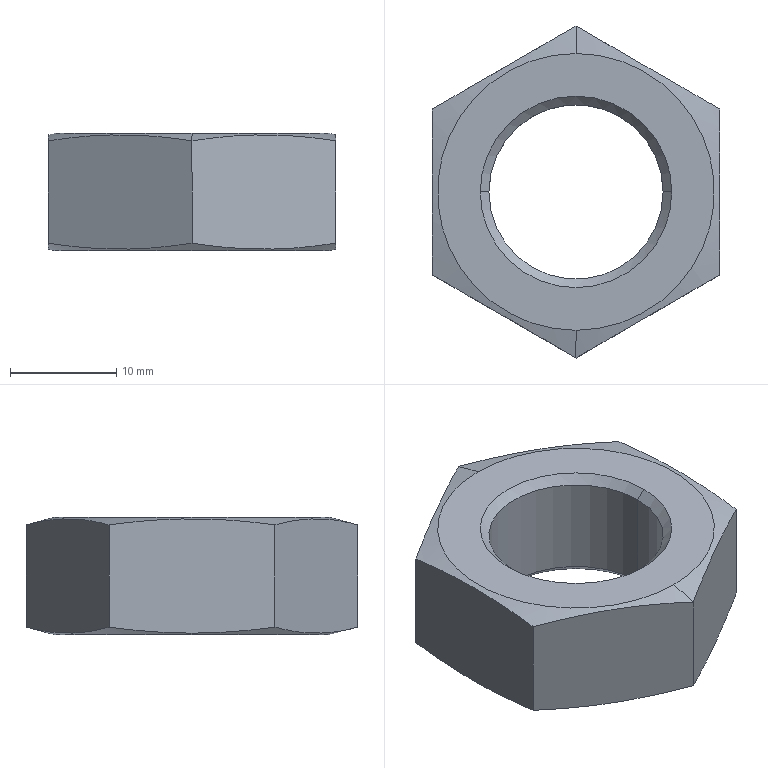Part | SolidWorks | features BaseBody 1 | 1 solid | 18 faces | box 27 x 31.177 x 11 mm | volume 4552 mm3 | cone 8 | plane 8 | cylinder 2 | commonest cylinder face diameters 16.376 x2
STEP:
#1=CARTESIAN_POINT('',(8.188,0.,4.688));
#2=VERTEX_POINT('',#1);
#3=CARTESIAN_POINT('',(-8.188,0.,4.688));
#4=VERTEX_POINT('',#3);
#5=CARTESIAN_POINT('',(0.,0.,4.688));
#6=DIRECTION('',(0.,0.,-1.));
#7=DIRECTION('',(-1.,0.,0.));
#8=AXIS2_PLACEMENT_3D('',#5,#6,#7);
#9=CIRCLE('',#8,8.188);
#10=EDGE_CURVE('',#2,#4,#9,.T.);
#11=ORIENTED_EDGE('',*,*,#10,.F.);
#12=CARTESIAN_POINT('',(8.188,0.,-4.688));
#13=VERTEX_POINT('',#12);
#14=CARTESIAN_POINT('',(8.188,0.,-5.5));
#15=DIRECTION('',(0.,0.,-1.));
#16=VECTOR('',#15,1000.);
#17=LINE('',#14,#16);
#18=EDGE_CURVE('',#2,#13,#17,.T.);
#19=ORIENTED_EDGE('',*,*,#18,.T.);
#20=CARTESIAN_POINT('',(-8.188,0.,-4.688));
#21=VERTEX_POINT('',#20);
#22=CARTESIAN_POINT('',(0.,0.,-4.688));
#23=DIRECTION('',(0.,0.,1.));
#24=DIRECTION('',(-1.,0.,0.));
#25=AXIS2_PLACEMENT_3D('',#22,#23,#24);
#26=CIRCLE('',#25,8.188);
#27=EDGE_CURVE('',#21,#13,#26,.T.);
#28=ORIENTED_EDGE('',*,*,#27,.F.);
#29=CARTESIAN_POINT('',(-8.188,0.,-5.5));
#30=DIRECTION('',(0.,0.,-1.));
#31=VECTOR('',#30,1000.);
#32=LINE('',#29,#31);
#33=EDGE_CURVE('',#4,#21,#32,.T.);
#34=ORIENTED_EDGE('',*,*,#33,.F.);
#35=EDGE_LOOP('',(#11,#19,#28,#34));
#36=FACE_OUTER_BOUND('',#35,.T.);
#37=CARTESIAN_POINT('',(0.,0.,-5.5));
#38=DIRECTION('',(0.,0.,-1.));
#39=DIRECTION('',(-1.,0.,0.));
#40=AXIS2_PLACEMENT_3D('',#37,#38,#39);
#41=CYLINDRICAL_SURFACE('',#40,8.188);
#42=ADVANCED_FACE('',(#36),#41,.F.);
#43=ORIENTED_EDGE('',*,*,#10,.T.);
#44=CARTESIAN_POINT('',(-9.,0.,5.5));
#45=VERTEX_POINT('',#44);
#46=CARTESIAN_POINT('',(-9.,0.,5.5));
#47=DIRECTION('',(-0.7071,0.,0.7071));
#48=VECTOR('',#47,1000.);
#49=LINE('',#46,#48);
#50=EDGE_CURVE('',#4,#45,#49,.T.);
#51=ORIENTED_EDGE('',*,*,#50,.T.);
#52=CARTESIAN_POINT('',(9.,0.,5.5));
#53=VERTEX_POINT('',#52);
#54=CARTESIAN_POINT('',(0.,0.,5.5));
#55=DIRECTION('',(0.,0.,-1.));
#56=DIRECTION('',(1.,0.,0.));
#57=AXIS2_PLACEMENT_3D('',#54,#55,#56);
#58=CIRCLE('',#57,9.);
#59=EDGE_CURVE('',#53,#45,#58,.T.);
#60=ORIENTED_EDGE('',*,*,#59,.F.);
#61=CARTESIAN_POINT('',(9.,0.,5.5));
#62=DIRECTION('',(0.7071,0.,0.7071));
#63=VECTOR('',#62,1000.);
#64=LINE('',#61,#63);
#65=EDGE_CURVE('',#2,#53,#64,.T.);
#66=ORIENTED_EDGE('',*,*,#65,.F.);
#67=EDGE_LOOP('',(#43,#51,#60,#66));
#68=FACE_OUTER_BOUND('',#67,.T.);
#69=CARTESIAN_POINT('',(0.,0.,5.5));
#70=DIRECTION('',(0.,0.,1.));
#71=DIRECTION('',(1.,0.,0.));
#72=AXIS2_PLACEMENT_3D('',#69,#70,#71);
#73=CONICAL_SURFACE('',#72,9.,0.7854);
#74=ADVANCED_FACE('',(#68),#73,.F.);
#75=ORIENTED_EDGE('',*,*,#27,.T.);
#76=CARTESIAN_POINT('',(9.,0.,-5.5));
#77=VERTEX_POINT('',#76);
#78=CARTESIAN_POINT('',(9.,0.,-5.5));
#79=DIRECTION('',(0.7071,0.,-0.7071));
#80=VECTOR('',#79,1000.);
#81=LINE('',#78,#80);
#82=EDGE_CURVE('',#13,#77,#81,.T.);
#83=ORIENTED_EDGE('',*,*,#82,.T.);
#84=CARTESIAN_POINT('',(-9.,0.,-5.5));
#85=VERTEX_POINT('',#84);
#86=CARTESIAN_POINT('',(0.,0.,-5.5));
#87=DIRECTION('',(0.,0.,1.));
#88=DIRECTION('',(-1.,0.,0.));
#89=AXIS2_PLACEMENT_3D('',#86,#87,#88);
#90=CIRCLE('',#89,9.);
#91=EDGE_CURVE('',#85,#77,#90,.T.);
#92=ORIENTED_EDGE('',*,*,#91,.F.);
#93=CARTESIAN_POINT('',(-9.,0.,-5.5));
#94=DIRECTION('',(-0.7071,0.,-0.7071));
#95=VECTOR('',#94,1000.);
#96=LINE('',#93,#95);
#97=EDGE_CURVE('',#21,#85,#96,.T.);
#98=ORIENTED_EDGE('',*,*,#97,.F.);
#99=EDGE_LOOP('',(#75,#83,#92,#98));
#100=FACE_OUTER_BOUND('',#99,.T.);
#101=CARTESIAN_POINT('',(0.,0.,-5.5));
#102=DIRECTION('',(0.,0.,-1.));
#103=DIRECTION('',(-1.,0.,0.));
#104=AXIS2_PLACEMENT_3D('',#101,#102,#103);
#105=CONICAL_SURFACE('',#104,9.,0.7854);
#106=ADVANCED_FACE('',(#100),#105,.F.);
#107=CARTESIAN_POINT('',(0.,-13.,5.5));
#108=VERTEX_POINT('',#107);
#109=CARTESIAN_POINT('',(0.,13.,5.5));
#110=VERTEX_POINT('',#109);
#111=CARTESIAN_POINT('',(0.,0.,5.5));
#112=DIRECTION('',(0.,0.,1.));
#113=DIRECTION('',(0.,1.,0.));
#114=AXIS2_PLACEMENT_3D('',#111,#112,#113);
#115=CIRCLE('',#114,13.);
#116=EDGE_CURVE('',#108,#110,#115,.T.);
#117=ORIENTED_EDGE('',*,*,#116,.F.);
#118=CARTESIAN_POINT('',(-0.000000051,-15.588,4.806));
#119=VERTEX_POINT('',#118);
#120=CARTESIAN_POINT('',(0.,-15.604,4.802));
#121=DIRECTION('',(0.,-0.9659,-0.2588));
#122=VECTOR('',#121,1000.);
#123=LINE('',#120,#122);
#124=EDGE_CURVE('',#108,#119,#123,.T.);
#125=ORIENTED_EDGE('',*,*,#124,.T.);
#126=CARTESIAN_POINT('',(13.5,-7.794,4.806));
#127=VERTEX_POINT('',#126);
#128=CARTESIAN_POINT('',(-0.000000051,-15.588,4.806));
#129=CARTESIAN_POINT('',(1.125,-14.939,4.98));
#130=CARTESIAN_POINT('',(2.25,-14.289,5.122));
#131=CARTESIAN_POINT('',(4.5,-12.99,5.315));
#132=CARTESIAN_POINT('',(6.75,-11.691,5.417));
#133=CARTESIAN_POINT('',(9.,-10.392,5.315));
#134=CARTESIAN_POINT('',(11.25,-9.093,5.122));
#135=CARTESIAN_POINT('',(12.375,-8.444,4.98));
#136=CARTESIAN_POINT('',(13.5,-7.794,4.806));
#137=B_SPLINE_CURVE_WITH_KNOTS('',3,(#128,#129,#130,#131,#132,#133,#134,#135,#136),.UNSPECIFIED.,.F.,.F.,(4,2,1,2,4),(0.,0.003897,0.007794,0.01169,0.01559),.UNSPECIFIED.);
#138=EDGE_CURVE('',#119,#127,#137,.T.);
#139=ORIENTED_EDGE('',*,*,#138,.T.);
#140=CARTESIAN_POINT('',(13.5,7.794,4.806));
#141=VERTEX_POINT('',#140);
#142=CARTESIAN_POINT('',(13.5,-7.794,4.806));
#143=CARTESIAN_POINT('',(13.5,-6.495,4.98));
#144=CARTESIAN_POINT('',(13.5,-5.196,5.122));
#145=CARTESIAN_POINT('',(13.5,-2.598,5.315));
#146=CARTESIAN_POINT('',(13.5,-0.000000076,5.417));
#147=CARTESIAN_POINT('',(13.5,2.598,5.315));
#148=CARTESIAN_POINT('',(13.5,5.196,5.122));
#149=CARTESIAN_POINT('',(13.5,6.495,4.98));
#150=CARTESIAN_POINT('',(13.5,7.794,4.806));
#151=B_SPLINE_CURVE_WITH_KNOTS('',3,(#142,#143,#144,#145,#146,#147,#148,#149,#150),.UNSPECIFIED.,.F.,.F.,(4,2,1,2,4),(0.,0.003897,0.007794,0.01169,0.01559),.UNSPECIFIED.);
#152=EDGE_CURVE('',#127,#141,#151,.T.);
#153=ORIENTED_EDGE('',*,*,#152,.T.);
#154=CARTESIAN_POINT('',(0.000000006,15.588,4.806));
#155=VERTEX_POINT('',#154);
#156=CARTESIAN_POINT('',(13.5,7.794,4.806));
#157=CARTESIAN_POINT('',(12.375,8.444,4.98));
#158=CARTESIAN_POINT('',(11.25,9.093,5.122));
#159=CARTESIAN_POINT('',(9.,10.392,5.315));
#160=CARTESIAN_POINT('',(6.75,11.691,5.417));
#161=CARTESIAN_POINT('',(4.5,12.99,5.315));
#162=CARTESIAN_POINT('',(2.25,14.289,5.122));
#163=CARTESIAN_POINT('',(1.125,14.939,4.98));
#164=CARTESIAN_POINT('',(0.000000006,15.588,4.806));
#165=B_SPLINE_CURVE_WITH_KNOTS('',3,(#156,#157,#158,#159,#160,#161,#162,#163,#164),.UNSPECIFIED.,.F.,.F.,(4,2,1,2,4),(0.,0.003897,0.007794,0.01169,0.01559),.UNSPECIFIED.);
#166=EDGE_CURVE('',#141,#155,#165,.T.);
#167=ORIENTED_EDGE('',*,*,#166,.T.);
#168=CARTESIAN_POINT('',(0.,15.604,4.802));
#169=DIRECTION('',(0.,0.9659,-0.2588));
#170=VECTOR('',#169,1000.);
#171=LINE('',#168,#170);
#172=EDGE_CURVE('',#110,#155,#171,.T.);
#173=ORIENTED_EDGE('',*,*,#172,.F.);
#174=EDGE_LOOP('',(#117,#125,#139,#153,#167,#173));
#175=FACE_OUTER_BOUND('',#174,.T.);
#176=CARTESIAN_POINT('',(0.,0.,4.802));
#177=DIRECTION('',(0.,0.,-1.));
#178=DIRECTION('',(0.,1.,0.));
#179=AXIS2_PLACEMENT_3D('',#176,#177,#178);
#180=CONICAL_SURFACE('',#179,15.604,1.309);
#181=ADVANCED_FACE('',(#175),#180,.T.);
#182=CARTESIAN_POINT('',(-13.,0.,-5.5));
#183=VERTEX_POINT('',#182);
#184=CARTESIAN_POINT('',(13.,0.,-5.5));
#185=VERTEX_POINT('',#184);
#186=CARTESIAN_POINT('',(0.,0.,-5.5));
#187=DIRECTION('',(0.,0.,-1.));
#188=DIRECTION('',(1.,0.,0.));
#189=AXIS2_PLACEMENT_3D('',#186,#187,#188);
#190=CIRCLE('',#189,13.);
#191=EDGE_CURVE('',#183,#185,#190,.T.);
#192=ORIENTED_EDGE('',*,*,#191,.F.);
#193=CARTESIAN_POINT('',(-13.5,0.,-5.366));
#194=VERTEX_POINT('',#193);
#195=CARTESIAN_POINT('',(-15.604,0.,-4.802));
#196=DIRECTION('',(-0.9659,0.,0.2588));
#197=VECTOR('',#196,1000.);
#198=LINE('',#195,#197);
#199=EDGE_CURVE('',#183,#194,#198,.T.);
#200=ORIENTED_EDGE('',*,*,#199,.T.);
#201=CARTESIAN_POINT('',(-13.5,7.794,-4.806));
#202=VERTEX_POINT('',#201);
#203=CARTESIAN_POINT('',(-13.5,0.,-5.366));
#204=CARTESIAN_POINT('',(-13.5,1.299,-5.366));
#205=CARTESIAN_POINT('',(-13.5,2.598,-5.315));
#206=CARTESIAN_POINT('',(-13.5,5.196,-5.122));
#207=CARTESIAN_POINT('',(-13.5,6.495,-4.98));
#208=CARTESIAN_POINT('',(-13.5,7.794,-4.806));
#209=B_SPLINE_CURVE_WITH_KNOTS('',3,(#203,#204,#205,#206,#207,#208),.UNSPECIFIED.,.F.,.F.,(4,2,4),(0.007794,0.01169,0.01559),.UNSPECIFIED.);
#210=EDGE_CURVE('',#194,#202,#209,.T.);
#211=ORIENTED_EDGE('',*,*,#210,.T.);
#212=CARTESIAN_POINT('',(-0.000000051,15.588,-4.806));
#213=VERTEX_POINT('',#212);
#214=CARTESIAN_POINT('',(-13.5,7.794,-4.806));
#215=CARTESIAN_POINT('',(-12.375,8.444,-4.98));
#216=CARTESIAN_POINT('',(-11.25,9.093,-5.122));
#217=CARTESIAN_POINT('',(-9.,10.392,-5.315));
#218=CARTESIAN_POINT('',(-6.75,11.691,-5.417));
#219=CARTESIAN_POINT('',(-4.5,12.99,-5.315));
#220=CARTESIAN_POINT('',(-2.25,14.289,-5.122));
#221=CARTESIAN_POINT('',(-1.125,14.939,-4.98));
#222=CARTESIAN_POINT('',(-0.000000051,15.588,-4.806));
#223=B_SPLINE_CURVE_WITH_KNOTS('',3,(#214,#215,#216,#217,#218,#219,#220,#221,#222),.UNSPECIFIED.,.F.,.F.,(4,2,1,2,4),(0.,0.003897,0.007794,0.01169,0.01559),.UNSPECIFIED.);
#224=EDGE_CURVE('',#202,#213,#223,.T.);
#225=ORIENTED_EDGE('',*,*,#224,.T.);
#226=CARTESIAN_POINT('',(13.5,7.794,-4.806));
#227=VERTEX_POINT('',#226);
#228=CARTESIAN_POINT('',(-0.000000051,15.588,-4.806));
#229=CARTESIAN_POINT('',(1.125,14.939,-4.98));
#230=CARTESIAN_POINT('',(2.25,14.289,-5.122));
#231=CARTESIAN_POINT('',(4.5,12.99,-5.315));
#232=CARTESIAN_POINT('',(6.75,11.691,-5.417));
#233=CARTESIAN_POINT('',(9.,10.392,-5.315));
#234=CARTESIAN_POINT('',(11.25,9.093,-5.122));
#235=CARTESIAN_POINT('',(12.375,8.444,-4.98));
#236=CARTESIAN_POINT('',(13.5,7.794,-4.806));
#237=B_SPLINE_CURVE_WITH_KNOTS('',3,(#228,#229,#230,#231,#232,#233,#234,#235,#236),.UNSPECIFIED.,.F.,.F.,(4,2,1,2,4),(0.,0.003897,0.007794,0.01169,0.01559),.UNSPECIFIED.);
#238=EDGE_CURVE('',#213,#227,#237,.T.);
#239=ORIENTED_EDGE('',*,*,#238,.T.);
#240=CARTESIAN_POINT('',(13.5,0.,-5.366));
#241=VERTEX_POINT('',#240);
#242=CARTESIAN_POINT('',(13.5,7.794,-4.806));
#243=CARTESIAN_POINT('',(13.5,6.495,-4.98));
#244=CARTESIAN_POINT('',(13.5,5.196,-5.122));
#245=CARTESIAN_POINT('',(13.5,2.598,-5.315));
#246=CARTESIAN_POINT('',(13.5,1.299,-5.366));
#247=CARTESIAN_POINT('',(13.5,0.,-5.366));
#248=B_SPLINE_CURVE_WITH_KNOTS('',3,(#242,#243,#244,#245,#246,#247),.UNSPECIFIED.,.F.,.F.,(4,2,4),(0.,0.003897,0.007794),.UNSPECIFIED.);
#249=EDGE_CURVE('',#227,#241,#248,.T.);
#250=ORIENTED_EDGE('',*,*,#249,.T.);
#251=CARTESIAN_POINT('',(15.604,0.,-4.802));
#252=DIRECTION('',(0.9659,0.,0.2588));
#253=VECTOR('',#252,1000.);
#254=LINE('',#251,#253);
#255=EDGE_CURVE('',#185,#241,#254,.T.);
#256=ORIENTED_EDGE('',*,*,#255,.F.);
#257=EDGE_LOOP('',(#192,#200,#211,#225,#239,#250,#256));
#258=FACE_OUTER_BOUND('',#257,.T.);
#259=CARTESIAN_POINT('',(0.,0.,-4.802));
#260=DIRECTION('',(0.,0.,1.));
#261=DIRECTION('',(1.,0.,0.));
#262=AXIS2_PLACEMENT_3D('',#259,#260,#261);
#263=CONICAL_SURFACE('',#262,15.604,1.309);
#264=ADVANCED_FACE('',(#258),#263,.T.);
#265=ORIENTED_EDGE('',*,*,#18,.F.);
#266=CARTESIAN_POINT('',(0.,0.,4.688));
#267=DIRECTION('',(0.,0.,-1.));
#268=DIRECTION('',(-1.,0.,0.));
#269=AXIS2_PLACEMENT_3D('',#266,#267,#268);
#270=CIRCLE('',#269,8.188);
#271=EDGE_CURVE('',#4,#2,#270,.T.);
#272=ORIENTED_EDGE('',*,*,#271,.F.);
#273=ORIENTED_EDGE('',*,*,#33,.T.);
#274=CARTESIAN_POINT('',(0.,0.,-4.688));
#275=DIRECTION('',(0.,0.,1.));
#276=DIRECTION('',(-1.,0.,0.));
#277=AXIS2_PLACEMENT_3D('',#274,#275,#276);
#278=CIRCLE('',#277,8.188);
#279=EDGE_CURVE('',#13,#21,#278,.T.);
#280=ORIENTED_EDGE('',*,*,#279,.F.);
#281=EDGE_LOOP('',(#265,#272,#273,#280));
#282=FACE_OUTER_BOUND('',#281,.T.);
#283=CARTESIAN_POINT('',(0.,0.,-5.5));
#284=DIRECTION('',(0.,0.,-1.));
#285=DIRECTION('',(-1.,0.,0.));
#286=AXIS2_PLACEMENT_3D('',#283,#284,#285);
#287=CYLINDRICAL_SURFACE('',#286,8.188);
#288=ADVANCED_FACE('',(#282),#287,.F.);
#289=ORIENTED_EDGE('',*,*,#50,.F.);
#290=ORIENTED_EDGE('',*,*,#271,.T.);
#291=ORIENTED_EDGE('',*,*,#65,.T.);
#292=CARTESIAN_POINT('',(0.,0.,5.5));
#293=DIRECTION('',(0.,0.,-1.));
#294=DIRECTION('',(1.,0.,0.));
#295=AXIS2_PLACEMENT_3D('',#292,#293,#294);
#296=CIRCLE('',#295,9.);
#297=EDGE_CURVE('',#45,#53,#296,.T.);
#298=ORIENTED_EDGE('',*,*,#297,.F.);
#299=EDGE_LOOP('',(#289,#290,#291,#298));
#300=FACE_OUTER_BOUND('',#299,.T.);
#301=CARTESIAN_POINT('',(0.,0.,5.5));
#302=DIRECTION('',(0.,0.,1.));
#303=DIRECTION('',(1.,0.,0.));
#304=AXIS2_PLACEMENT_3D('',#301,#302,#303);
#305=CONICAL_SURFACE('',#304,9.,0.7854);
#306=ADVANCED_FACE('',(#300),#305,.F.);
#307=ORIENTED_EDGE('',*,*,#82,.F.);
#308=ORIENTED_EDGE('',*,*,#279,.T.);
#309=ORIENTED_EDGE('',*,*,#97,.T.);
#310=CARTESIAN_POINT('',(0.,0.,-5.5));
#311=DIRECTION('',(0.,0.,1.));
#312=DIRECTION('',(-1.,0.,0.));
#313=AXIS2_PLACEMENT_3D('',#310,#311,#312);
#314=CIRCLE('',#313,9.);
#315=EDGE_CURVE('',#77,#85,#314,.T.);
#316=ORIENTED_EDGE('',*,*,#315,.F.);
#317=EDGE_LOOP('',(#307,#308,#309,#316));
#318=FACE_OUTER_BOUND('',#317,.T.);
#319=CARTESIAN_POINT('',(0.,0.,-5.5));
#320=DIRECTION('',(0.,0.,-1.));
#321=DIRECTION('',(-1.,0.,0.));
#322=AXIS2_PLACEMENT_3D('',#319,#320,#321);
#323=CONICAL_SURFACE('',#322,9.,0.7854);
#324=ADVANCED_FACE('',(#318),#323,.F.);
#325=CARTESIAN_POINT('',(0.,0.,5.5));
#326=DIRECTION('',(0.,0.,1.));
#327=DIRECTION('',(0.,1.,0.));
#328=AXIS2_PLACEMENT_3D('',#325,#326,#327);
#329=CIRCLE('',#328,13.);
#330=EDGE_CURVE('',#110,#108,#329,.T.);
#331=ORIENTED_EDGE('',*,*,#330,.T.);
#332=ORIENTED_EDGE('',*,*,#116,.T.);
#333=EDGE_LOOP('',(#331,#332));
#334=FACE_OUTER_BOUND('',#333,.T.);
#335=ORIENTED_EDGE('',*,*,#59,.T.);
#336=ORIENTED_EDGE('',*,*,#297,.T.);
#337=EDGE_LOOP('',(#335,#336));
#338=FACE_BOUND('',#337,.T.);
#339=CARTESIAN_POINT('',(0.,13.,5.5));
#340=DIRECTION('',(0.,0.,1.));
#341=DIRECTION('',(1.,0.,0.));
#342=AXIS2_PLACEMENT_3D('',#339,#340,#341);
#343=PLANE('',#342);
#344=ADVANCED_FACE('',(#334,#338),#343,.T.);
#345=ORIENTED_EDGE('',*,*,#91,.T.);
#346=ORIENTED_EDGE('',*,*,#315,.T.);
#347=EDGE_LOOP('',(#345,#346));
#348=FACE_BOUND('',#347,.T.);
#349=CARTESIAN_POINT('',(0.,0.,-5.5));
#350=DIRECTION('',(0.,0.,-1.));
#351=DIRECTION('',(1.,0.,0.));
#352=AXIS2_PLACEMENT_3D('',#349,#350,#351);
#353=CIRCLE('',#352,13.);
#354=EDGE_CURVE('',#185,#183,#353,.T.);
#355=ORIENTED_EDGE('',*,*,#354,.T.);
#356=ORIENTED_EDGE('',*,*,#191,.T.);
#357=EDGE_LOOP('',(#355,#356));
#358=FACE_OUTER_BOUND('',#357,.T.);
#359=CARTESIAN_POINT('',(0.,9.,-5.5));
#360=DIRECTION('',(0.,0.,-1.));
#361=DIRECTION('',(-1.,0.,0.));
#362=AXIS2_PLACEMENT_3D('',#359,#360,#361);
#363=PLANE('',#362);
#364=ADVANCED_FACE('',(#348,#358),#363,.T.);
#365=ORIENTED_EDGE('',*,*,#124,.F.);
#366=ORIENTED_EDGE('',*,*,#330,.F.);
#367=ORIENTED_EDGE('',*,*,#172,.T.);
#368=CARTESIAN_POINT('',(-13.5,7.794,4.806));
#369=VERTEX_POINT('',#368);
#370=CARTESIAN_POINT('',(0.000000006,15.588,4.806));
#371=CARTESIAN_POINT('',(-1.125,14.939,4.98));
#372=CARTESIAN_POINT('',(-2.25,14.289,5.122));
#373=CARTESIAN_POINT('',(-4.5,12.99,5.315));
#374=CARTESIAN_POINT('',(-6.75,11.691,5.417));
#375=CARTESIAN_POINT('',(-9.,10.392,5.315));
#376=CARTESIAN_POINT('',(-11.25,9.093,5.122));
#377=CARTESIAN_POINT('',(-12.375,8.444,4.98));
#378=CARTESIAN_POINT('',(-13.5,7.794,4.806));
#379=B_SPLINE_CURVE_WITH_KNOTS('',3,(#370,#371,#372,#373,#374,#375,#376,#377,#378),.UNSPECIFIED.,.F.,.F.,(4,2,1,2,4),(0.,0.003897,0.007794,0.01169,0.01559),.UNSPECIFIED.);
#380=EDGE_CURVE('',#155,#369,#379,.T.);
#381=ORIENTED_EDGE('',*,*,#380,.T.);
#382=CARTESIAN_POINT('',(-13.5,-7.794,4.806));
#383=VERTEX_POINT('',#382);
#384=CARTESIAN_POINT('',(-13.5,7.794,4.806));
#385=CARTESIAN_POINT('',(-13.5,6.495,4.98));
#386=CARTESIAN_POINT('',(-13.5,5.196,5.122));
#387=CARTESIAN_POINT('',(-13.5,2.598,5.315));
#388=CARTESIAN_POINT('',(-13.5,0.,5.417));
#389=CARTESIAN_POINT('',(-13.5,-2.598,5.315));
#390=CARTESIAN_POINT('',(-13.5,-5.196,5.122));
#391=CARTESIAN_POINT('',(-13.5,-6.495,4.98));
#392=CARTESIAN_POINT('',(-13.5,-7.794,4.806));
#393=B_SPLINE_CURVE_WITH_KNOTS('',3,(#384,#385,#386,#387,#388,#389,#390,#391,#392),.UNSPECIFIED.,.F.,.F.,(4,2,1,2,4),(0.,0.003897,0.007794,0.01169,0.01559),.UNSPECIFIED.);
#394=EDGE_CURVE('',#369,#383,#393,.T.);
#395=ORIENTED_EDGE('',*,*,#394,.T.);
#396=CARTESIAN_POINT('',(-13.5,-7.794,4.806));
#397=CARTESIAN_POINT('',(-12.375,-8.444,4.98));
#398=CARTESIAN_POINT('',(-11.25,-9.093,5.122));
#399=CARTESIAN_POINT('',(-9.,-10.392,5.315));
#400=CARTESIAN_POINT('',(-6.75,-11.691,5.417));
#401=CARTESIAN_POINT('',(-4.5,-12.99,5.315));
#402=CARTESIAN_POINT('',(-2.25,-14.289,5.122));
#403=CARTESIAN_POINT('',(-1.125,-14.939,4.98));
#404=CARTESIAN_POINT('',(-0.000000051,-15.588,4.806));
#405=B_SPLINE_CURVE_WITH_KNOTS('',3,(#396,#397,#398,#399,#400,#401,#402,#403,#404),.UNSPECIFIED.,.F.,.F.,(4,2,1,2,4),(0.,0.003897,0.007794,0.01169,0.01559),.UNSPECIFIED.);
#406=EDGE_CURVE('',#383,#119,#405,.T.);
#407=ORIENTED_EDGE('',*,*,#406,.T.);
#408=EDGE_LOOP('',(#365,#366,#367,#381,#395,#407));
#409=FACE_OUTER_BOUND('',#408,.T.);
#410=CARTESIAN_POINT('',(0.,0.,4.802));
#411=DIRECTION('',(0.,0.,-1.));
#412=DIRECTION('',(0.,1.,0.));
#413=AXIS2_PLACEMENT_3D('',#410,#411,#412);
#414=CONICAL_SURFACE('',#413,15.604,1.309);
#415=ADVANCED_FACE('',(#409),#414,.T.);
#416=ORIENTED_EDGE('',*,*,#199,.F.);
#417=ORIENTED_EDGE('',*,*,#354,.F.);
#418=ORIENTED_EDGE('',*,*,#255,.T.);
#419=CARTESIAN_POINT('',(13.5,-7.794,-4.806));
#420=VERTEX_POINT('',#419);
#421=CARTESIAN_POINT('',(13.5,0.,-5.366));
#422=CARTESIAN_POINT('',(13.5,-1.299,-5.366));
#423=CARTESIAN_POINT('',(13.5,-2.598,-5.315));
#424=CARTESIAN_POINT('',(13.5,-5.196,-5.122));
#425=CARTESIAN_POINT('',(13.5,-6.495,-4.98));
#426=CARTESIAN_POINT('',(13.5,-7.794,-4.806));
#427=B_SPLINE_CURVE_WITH_KNOTS('',3,(#421,#422,#423,#424,#425,#426),.UNSPECIFIED.,.F.,.F.,(4,2,4),(0.007794,0.01169,0.01559),.UNSPECIFIED.);
#428=EDGE_CURVE('',#241,#420,#427,.T.);
#429=ORIENTED_EDGE('',*,*,#428,.T.);
#430=CARTESIAN_POINT('',(0.000000051,-15.588,-4.806));
#431=VERTEX_POINT('',#430);
#432=CARTESIAN_POINT('',(13.5,-7.794,-4.806));
#433=CARTESIAN_POINT('',(12.375,-8.444,-4.98));
#434=CARTESIAN_POINT('',(11.25,-9.093,-5.122));
#435=CARTESIAN_POINT('',(9.,-10.392,-5.315));
#436=CARTESIAN_POINT('',(6.75,-11.691,-5.417));
#437=CARTESIAN_POINT('',(4.5,-12.99,-5.315));
#438=CARTESIAN_POINT('',(2.25,-14.289,-5.122));
#439=CARTESIAN_POINT('',(1.125,-14.939,-4.98));
#440=CARTESIAN_POINT('',(0.000000051,-15.588,-4.806));
#441=B_SPLINE_CURVE_WITH_KNOTS('',3,(#432,#433,#434,#435,#436,#437,#438,#439,#440),.UNSPECIFIED.,.F.,.F.,(4,2,1,2,4),(0.,0.003897,0.007794,0.01169,0.01559),.UNSPECIFIED.);
#442=EDGE_CURVE('',#420,#431,#441,.T.);
#443=ORIENTED_EDGE('',*,*,#442,.T.);
#444=CARTESIAN_POINT('',(-13.5,-7.794,-4.806));
#445=VERTEX_POINT('',#444);
#446=CARTESIAN_POINT('',(0.000000051,-15.588,-4.806));
#447=CARTESIAN_POINT('',(-1.125,-14.939,-4.98));
#448=CARTESIAN_POINT('',(-2.25,-14.289,-5.122));
#449=CARTESIAN_POINT('',(-4.5,-12.99,-5.315));
#450=CARTESIAN_POINT('',(-6.75,-11.691,-5.417));
#451=CARTESIAN_POINT('',(-9.,-10.392,-5.315));
#452=CARTESIAN_POINT('',(-11.25,-9.093,-5.122));
#453=CARTESIAN_POINT('',(-12.375,-8.444,-4.98));
#454=CARTESIAN_POINT('',(-13.5,-7.794,-4.806));
#455=B_SPLINE_CURVE_WITH_KNOTS('',3,(#446,#447,#448,#449,#450,#451,#452,#453,#454),.UNSPECIFIED.,.F.,.F.,(4,2,1,2,4),(0.,0.003897,0.007794,0.01169,0.01559),.UNSPECIFIED.);
#456=EDGE_CURVE('',#431,#445,#455,.T.);
#457=ORIENTED_EDGE('',*,*,#456,.T.);
#458=CARTESIAN_POINT('',(-13.5,-7.794,-4.806));
#459=CARTESIAN_POINT('',(-13.5,-6.495,-4.98));
#460=CARTESIAN_POINT('',(-13.5,-5.196,-5.122));
#461=CARTESIAN_POINT('',(-13.5,-2.598,-5.315));
#462=CARTESIAN_POINT('',(-13.5,-1.299,-5.366));
#463=CARTESIAN_POINT('',(-13.5,0.,-5.366));
#464=B_SPLINE_CURVE_WITH_KNOTS('',3,(#458,#459,#460,#461,#462,#463),.UNSPECIFIED.,.F.,.F.,(4,2,4),(0.,0.003897,0.007794),.UNSPECIFIED.);
#465=EDGE_CURVE('',#445,#194,#464,.T.);
#466=ORIENTED_EDGE('',*,*,#465,.T.);
#467=EDGE_LOOP('',(#416,#417,#418,#429,#443,#457,#466));
#468=FACE_OUTER_BOUND('',#467,.T.);
#469=CARTESIAN_POINT('',(0.,0.,-4.802));
#470=DIRECTION('',(0.,0.,1.));
#471=DIRECTION('',(1.,0.,0.));
#472=AXIS2_PLACEMENT_3D('',#469,#470,#471);
#473=CONICAL_SURFACE('',#472,15.604,1.309);
#474=ADVANCED_FACE('',(#468),#473,.T.);
#475=CARTESIAN_POINT('',(0.,15.588,5.5));
#476=DIRECTION('',(0.,0.,1.));
#477=VECTOR('',#476,1000.);
#478=LINE('',#475,#477);
#479=EDGE_CURVE('',#213,#155,#478,.T.);
#480=ORIENTED_EDGE('',*,*,#479,.F.);
#481=ORIENTED_EDGE('',*,*,#224,.F.);
#482=CARTESIAN_POINT('',(-13.5,7.794,5.5));
#483=DIRECTION('',(0.,0.,-1.));
#484=VECTOR('',#483,1000.);
#485=LINE('',#482,#484);
#486=EDGE_CURVE('',#369,#202,#485,.T.);
#487=ORIENTED_EDGE('',*,*,#486,.F.);
#488=ORIENTED_EDGE('',*,*,#380,.F.);
#489=EDGE_LOOP('',(#480,#481,#487,#488));
#490=FACE_OUTER_BOUND('',#489,.T.);
#491=CARTESIAN_POINT('',(0.,15.588,5.5));
#492=DIRECTION('',(0.5,-0.866,0.));
#493=DIRECTION('',(0.866,0.5,0.));
#494=AXIS2_PLACEMENT_3D('',#491,#492,#493);
#495=PLANE('',#494);
#496=ADVANCED_FACE('',(#490),#495,.F.);
#497=CARTESIAN_POINT('',(13.5,7.794,5.5));
#498=DIRECTION('',(0.,0.,1.));
#499=VECTOR('',#498,1000.);
#500=LINE('',#497,#499);
#501=EDGE_CURVE('',#227,#141,#500,.T.);
#502=ORIENTED_EDGE('',*,*,#501,.F.);
#503=ORIENTED_EDGE('',*,*,#238,.F.);
#504=ORIENTED_EDGE('',*,*,#479,.T.);
#505=ORIENTED_EDGE('',*,*,#166,.F.);
#506=EDGE_LOOP('',(#502,#503,#504,#505));
#507=FACE_OUTER_BOUND('',#506,.T.);
#508=CARTESIAN_POINT('',(13.5,7.794,5.5));
#509=DIRECTION('',(-0.5,-0.866,0.));
#510=DIRECTION('',(0.866,-0.5,0.));
#511=AXIS2_PLACEMENT_3D('',#508,#509,#510);
#512=PLANE('',#511);
#513=ADVANCED_FACE('',(#507),#512,.F.);
#514=CARTESIAN_POINT('',(13.5,-7.794,5.5));
#515=DIRECTION('',(0.,0.,1.));
#516=VECTOR('',#515,1000.);
#517=LINE('',#514,#516);
#518=EDGE_CURVE('',#420,#127,#517,.T.);
#519=ORIENTED_EDGE('',*,*,#518,.F.);
#520=ORIENTED_EDGE('',*,*,#428,.F.);
#521=ORIENTED_EDGE('',*,*,#249,.F.);
#522=ORIENTED_EDGE('',*,*,#501,.T.);
#523=ORIENTED_EDGE('',*,*,#152,.F.);
#524=EDGE_LOOP('',(#519,#520,#521,#522,#523));
#525=FACE_OUTER_BOUND('',#524,.T.);
#526=CARTESIAN_POINT('',(13.5,-7.794,5.5));
#527=DIRECTION('',(-1.,0.,0.));
#528=DIRECTION('',(0.,0.,1.));
#529=AXIS2_PLACEMENT_3D('',#526,#527,#528);
#530=PLANE('',#529);
#531=ADVANCED_FACE('',(#525),#530,.F.);
#532=CARTESIAN_POINT('',(0.,-15.588,5.5));
#533=DIRECTION('',(0.,0.,1.));
#534=VECTOR('',#533,1000.);
#535=LINE('',#532,#534);
#536=EDGE_CURVE('',#431,#119,#535,.T.);
#537=ORIENTED_EDGE('',*,*,#536,.F.);
#538=ORIENTED_EDGE('',*,*,#442,.F.);
#539=ORIENTED_EDGE('',*,*,#518,.T.);
#540=ORIENTED_EDGE('',*,*,#138,.F.);
#541=EDGE_LOOP('',(#537,#538,#539,#540));
#542=FACE_OUTER_BOUND('',#541,.T.);
#543=CARTESIAN_POINT('',(0.,-15.588,5.5));
#544=DIRECTION('',(-0.5,0.866,0.));
#545=DIRECTION('',(-0.866,-0.5,0.));
#546=AXIS2_PLACEMENT_3D('',#543,#544,#545);
#547=PLANE('',#546);
#548=ADVANCED_FACE('',(#542),#547,.F.);
#549=CARTESIAN_POINT('',(-13.5,-7.794,5.5));
#550=DIRECTION('',(0.,0.,1.));
#551=VECTOR('',#550,1000.);
#552=LINE('',#549,#551);
#553=EDGE_CURVE('',#445,#383,#552,.T.);
#554=ORIENTED_EDGE('',*,*,#553,.F.);
#555=ORIENTED_EDGE('',*,*,#456,.F.);
#556=ORIENTED_EDGE('',*,*,#536,.T.);
#557=ORIENTED_EDGE('',*,*,#406,.F.);
#558=EDGE_LOOP('',(#554,#555,#556,#557));
#559=FACE_OUTER_BOUND('',#558,.T.);
#560=CARTESIAN_POINT('',(-13.5,-7.794,5.5));
#561=DIRECTION('',(0.5,0.866,0.));
#562=DIRECTION('',(-0.866,0.5,0.));
#563=AXIS2_PLACEMENT_3D('',#560,#561,#562);
#564=PLANE('',#563);
#565=ADVANCED_FACE('',(#559),#564,.F.);
#566=ORIENTED_EDGE('',*,*,#486,.T.);
#567=ORIENTED_EDGE('',*,*,#210,.F.);
#568=ORIENTED_EDGE('',*,*,#465,.F.);
#569=ORIENTED_EDGE('',*,*,#553,.T.);
#570=ORIENTED_EDGE('',*,*,#394,.F.);
#571=EDGE_LOOP('',(#566,#567,#568,#569,#570));
#572=FACE_OUTER_BOUND('',#571,.T.);
#573=CARTESIAN_POINT('',(-13.5,7.794,5.5));
#574=DIRECTION('',(1.,0.,0.));
#575=DIRECTION('',(0.,0.,-1.));
#576=AXIS2_PLACEMENT_3D('',#573,#574,#575);
#577=PLANE('',#576);
#578=ADVANCED_FACE('',(#572),#577,.F.);
#579=CLOSED_SHELL('',(#42,#74,#106,#181,#264,#288,#306,#324,#344,#364,#415,#474,#496,#513,#531,#548,#565,#578));
#580=MANIFOLD_SOLID_BREP('',#579);
#581=CARTESIAN_POINT('',(0.,0.,0.));
#582=DIRECTION('',(0.,0.,1.));
#583=DIRECTION('',(1.,0.,0.));
#584=AXIS2_PLACEMENT_3D('',#581,#582,#583);
#585=(LENGTH_UNIT()NAMED_UNIT(*)SI_UNIT(.MILLI.,.METRE.));
#586=UNCERTAINTY_MEASURE_WITH_UNIT(LENGTH_MEASURE(0.00001),#585,'','');
#587=(NAMED_UNIT(*)PLANE_ANGLE_UNIT()SI_UNIT($,.RADIAN.));
#588=(NAMED_UNIT(*)SI_UNIT($,.STERADIAN.)SOLID_ANGLE_UNIT());
#589=(GEOMETRIC_REPRESENTATION_CONTEXT(3)GLOBAL_UNCERTAINTY_ASSIGNED_CONTEXT((#586))GLOBAL_UNIT_ASSIGNED_CONTEXT((#585,#587,#588))REPRESENTATION_CONTEXT('',''));
#590=ADVANCED_BREP_SHAPE_REPRESENTATION('',(#580,#584),#589);